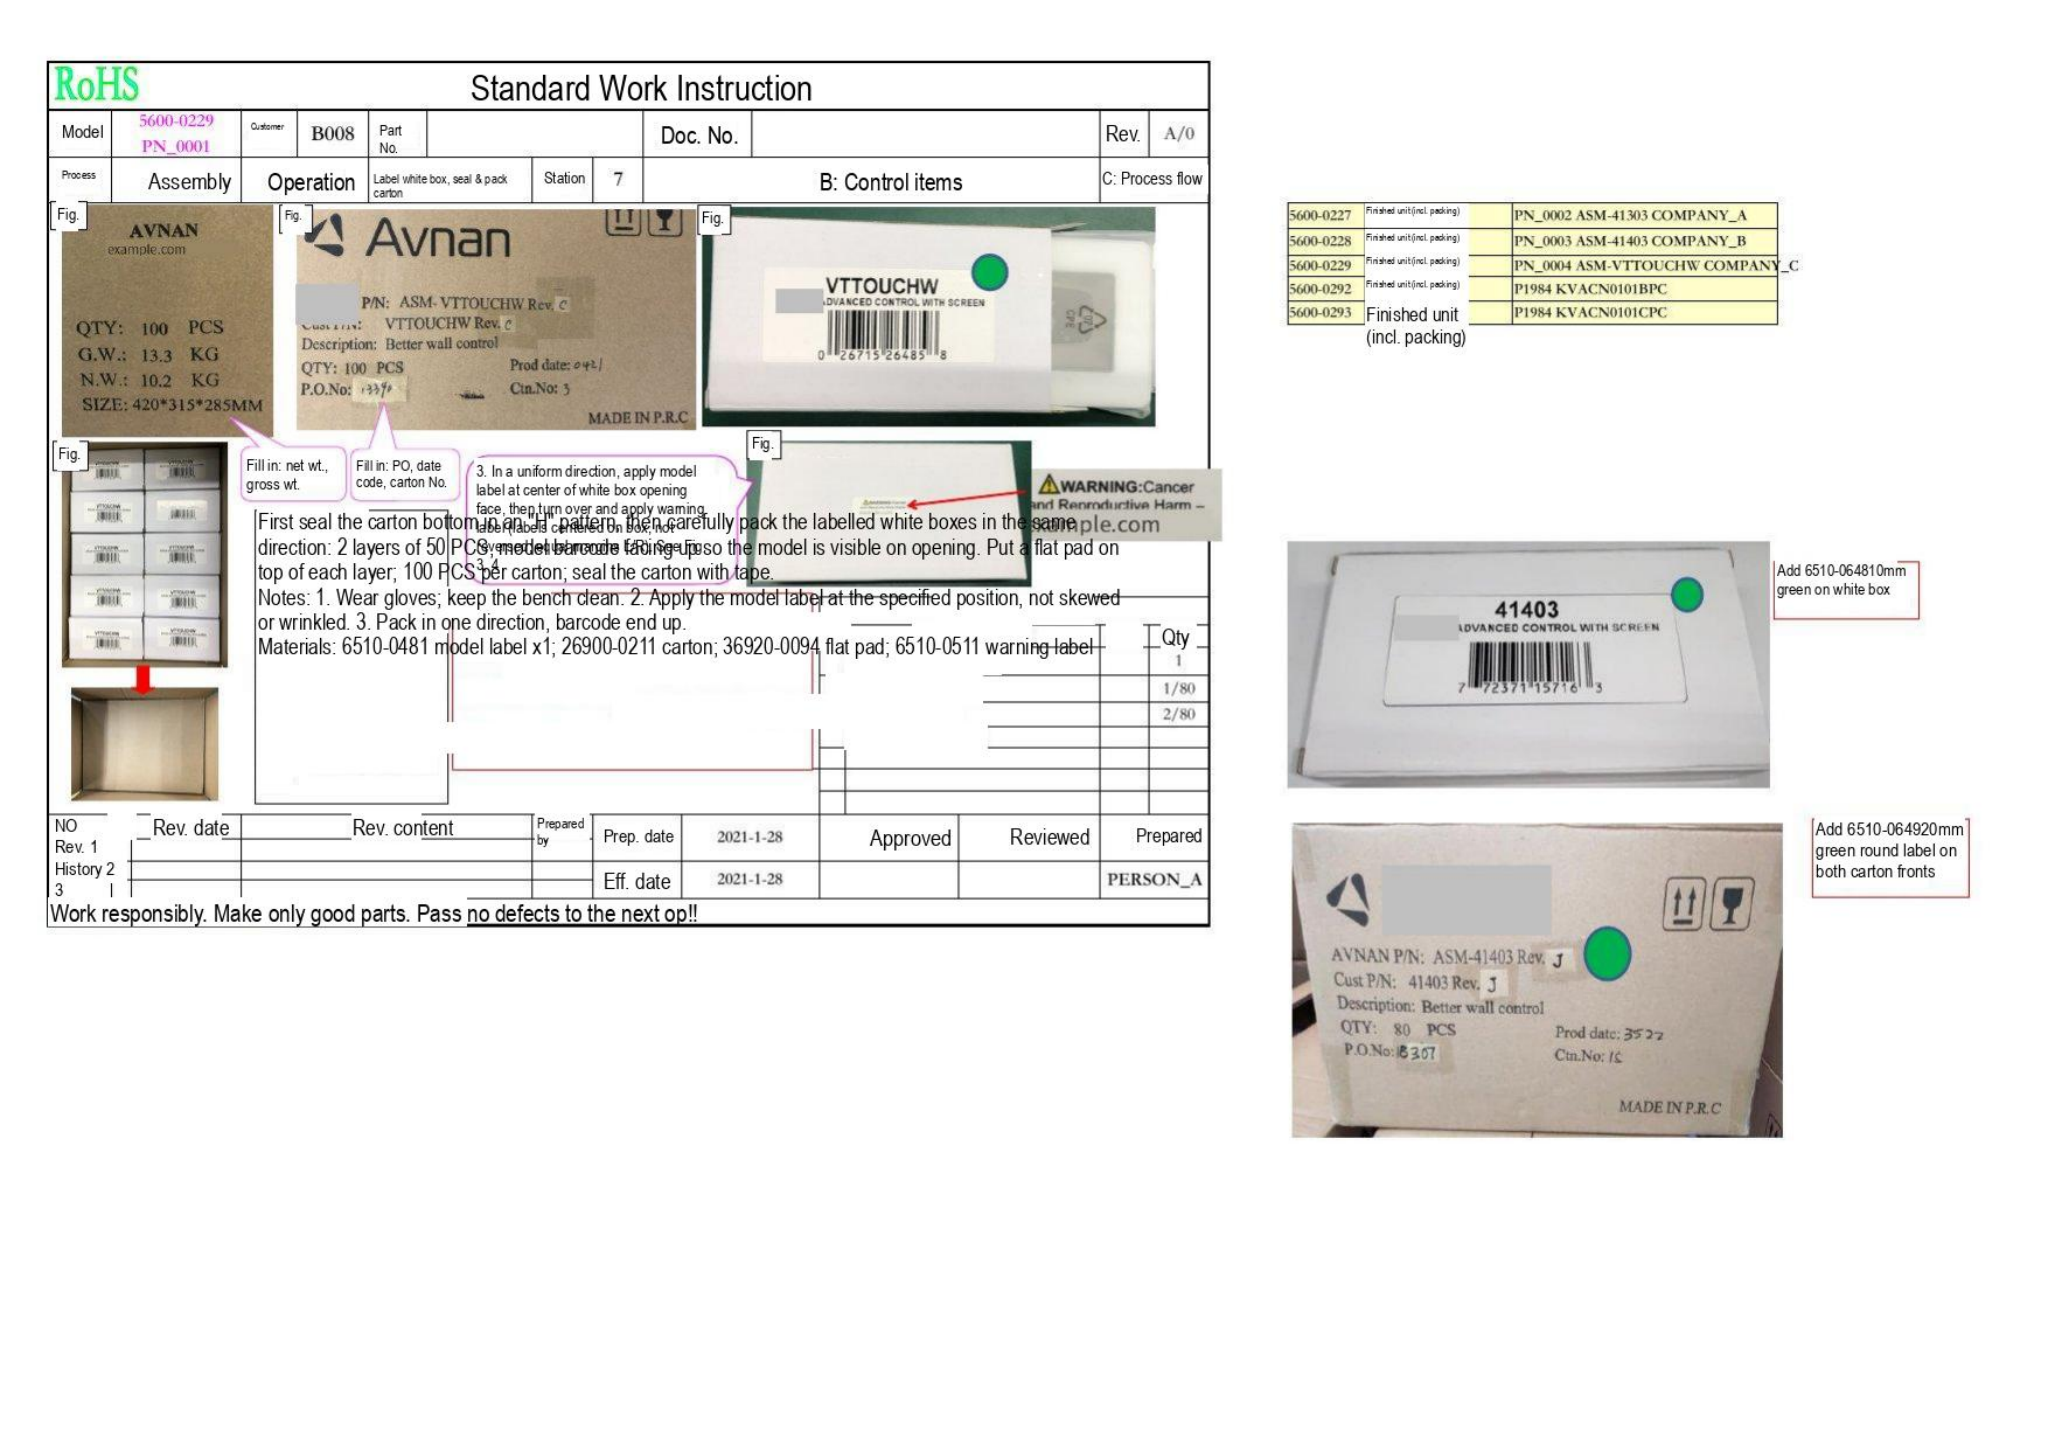RoHS

Standard Work Instruction

| Model | 5600-0229 PN_0001 | Customer | B008 | Part No. | | Doc. No. | | Rev. | A/0 |
|---|---|---|---|---|---|---|---|---|---|
| Process | Assembly | Operation | Label white box, seal & pack carton | Station | 7 | B: Control items | | C: Process flow | |

Fig.

AVNAN
example.com
QTY: 100 PCS
G.W.: 13.3 KG
N.W.: 10.2 KG
SIZE: 420*315*285MM

Fig.

Avnan
P/N: ASM-VTTOUCHW Rev. C
Cust P/N: VTTOUCHW Rev. C
Description: Better wall control
QTY: 100 PCS
P.O.No:
Prod date:
Ctn.No: 3
MADE IN P.R.C

Fig.

VTTOUCHW
ADVANCED CONTROL WITH SCREEN
0 26715 26485 8

Fig.

Fig.

WARNING: Cancer and Reproductive Harm – example.com

Fill in: net wt., gross wt.

Fill in: PO, date code, carton No.

3. In a uniform direction, apply model label at center of white box opening face, then turn over and apply warning label (labels centered on box, not skewed, model barcode facing up). See Fig. 3, 4

First seal the carton bottom in an "H" pattern, then carefully pack the labelled white boxes in the same direction: 2 layers of 50 PCS, model barcode facing up so the model is visible on opening. Put a flat pad on top of each layer; 100 PCS per carton; seal the carton with tape.
Notes: 1. Wear gloves; keep the bench clean. 2. Apply the model label at the specified position, not skewed or wrinkled. 3. Pack in one direction, barcode end up.
Materials: 6510-0481 model label x1; 26900-0211 carton; 36920-0094 flat pad; 6510-0511 warning label

| Qty |
|---|
| 1 |
| 1/80 |
| 2/80 |

| NO | Rev. date | Rev. content | Prepared by | Prep. date | 2021-1-28 | Approved | Reviewed | Prepared |
|---|---|---|---|---|---|---|---|---|
| Rev. 1 | | | | | | | | |
| History 2 | | | | | | | | |
| 3 | | | | Eff. date | 2021-1-28 | | | PERSON_A |

Work responsibly. Make only good parts. Pass no defects to the next op!!

| 5600-0227 | Finished unit (incl. packing) | PN_0002 ASM-41303 COMPANY_A |
|---|---|---|
| 5600-0228 | Finished unit (incl. packing) | PN_0003 ASM-41403 COMPANY_B |
| 5600-0229 | Finished unit (incl. packing) | PN_0004 ASM-VTTOUCHW COMPANY_C |
| 5600-0292 | Finished unit (incl. packing) | P1984 KVACN0101BPC |
| 5600-0293 | Finished unit (incl. packing) | P1984 KVACN0101CPC |

41403
ADVANCED CONTROL WITH SCREEN
7 72371 15716 3

Add 6510-064810mm green on white box

AVNAN P/N: ASM-41403 Rev. J
Cust P/N: 41403 Rev. J
Description: Better wall control
QTY: 80 PCS
P.O.No: 8307
Prod date: 3522
Ctn.No: 16
MADE IN P.R.C

Add 6510-064920mm green round label on both carton fronts